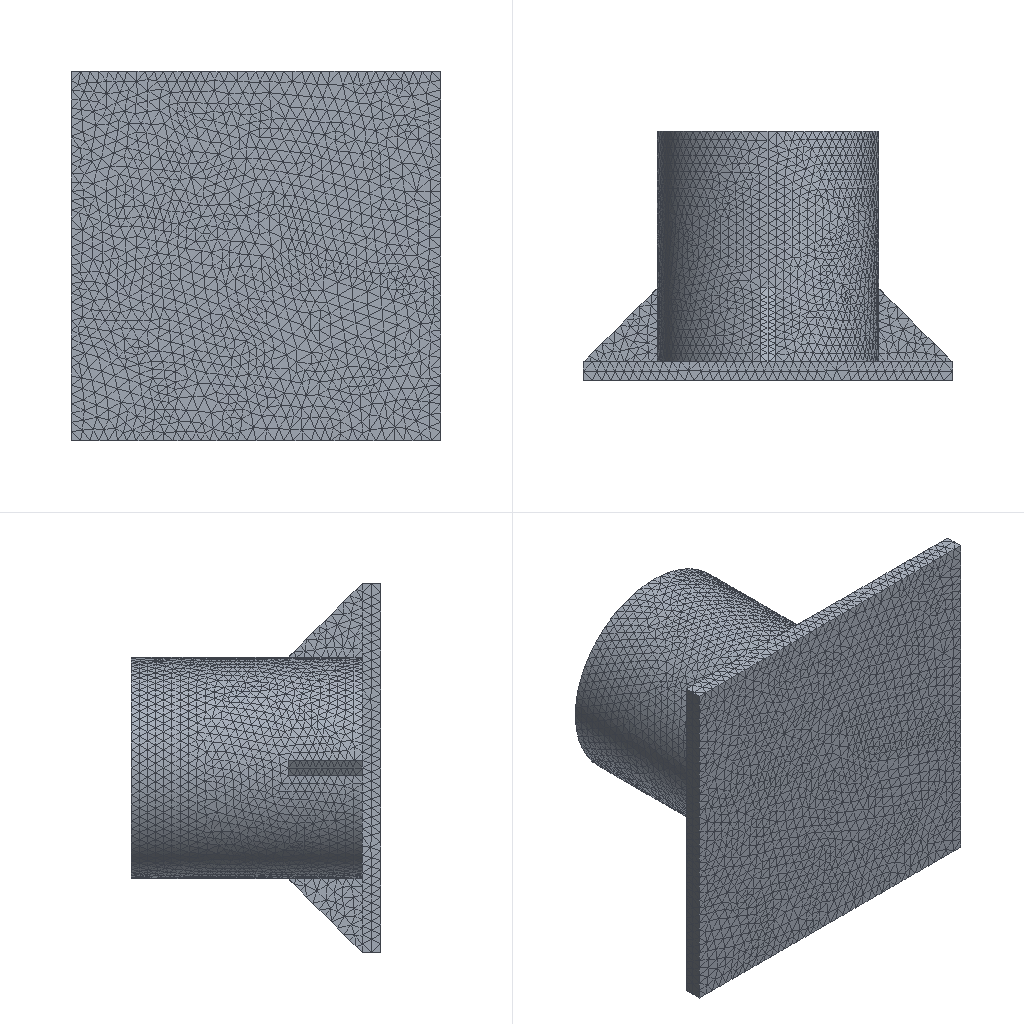Simulation study | ansys workbench
Set-up summary:
category,name,step,type,value,unit,region
solver,ansys_workbench
units,mm-N-s-tonne (MPa),,stated,"/units,MPA"
analysis,LS1,,modal,method=lanb; n_modes=3
load_step,LS1,LS1,modal
mesh,nodes,,,70254
mesh,elements,,,42512
element_type,SOLID187,,,41872
element_type,CONTA174,,,640
material,Structural Steel,,E,200000,tonne s^-2 mm^-1
material,Structural Steel,,nu,0.3
material,Structural Steel,,density,7.8e-09,tonne mm^-3
bc,Construct Remote Displacement,model,fixed,"[dofs=ROTX,ROTY,ROTZ,UX,UY,UZ n=20]",,node list
contact,contact 1,,bonded (always),element=CONTA174
contact,contact 2,,bonded (always),element=CONTA174
contact,contact 3,,bonded (always),element=CONTA174
contact,contact 4,,bonded (always),element=CONTA174
named_set,REMOTEDISPALL,,node,4
Ansys APDL input file, long lists of numbers shortened:
/batch
/config,noeldb,1     ! force off writing results to database
*get,_wallstrt,active,,time,wall
! ANSYS input file written by Workbench version 2021 R1
! File used for geometry attach:
/title,wbnew--__ (C5)
! ****** Begin Custom Load Command Snippet ******
/COM, ACT Extensions:
/COM,     LSDYNA, 2021.1
/COM,
! ****** End   Custom Load Command Snippet ******
*DIM,_wb_ProjectScratch_dir,string,248
_wb_ProjectScratch_dir(1) = ''
*DIM,_wb_SolverFiles_dir,string,248
_wb_SolverFiles_dir(1) = ''
*DIM,_wb_userfiles_dir,string,248
_wb_userfiles_dir(1) = ''
/com,--- Data in consistent NMM units. See Solving Units in the help system for more information.
/units,MPA
/nopr
/wb,file,start              !  signify a WB generated input file
/prep7
! Turn off shape checking because checks already performed inside WB mesher.
! See help system for more information.
SHPP,OFF,,NOWARN
/nolist
etcon,set             ! allow ANSYS to choose best KEYOP's for 180x elements, resets any applicable keyopt to MAPDL defaults
/com,*********** Nodes for the whole assembly ***********
nblock,3,,77270
(1i9,3e20.9e3)
        1     0.000000000E+00     2.700000000E+03    -1.000000000E+03
! (70245 more lines like these left out)
-1
/com,*********** Nodes for all Remote Points ***********
nblock,3
(1i9,3e20.9e3)
    70247    -2.000000000E+03     1.000000000E+02    -3.725290298E-14
! (7 more lines like these left out)
-1
/wb,elem,start            !  set before creation of elements
/com,*********** Elements for Body 1 "__-FreeParts|____(____)1" ***********
et,1,187
eblock,19,solid,,41872
(19i9)
        1        1        1        1        0        0        0        0       10        0        1     8226    10631     9051     9803    64966    68065    64961    64962
! (83743 more lines like these left out)
-1
/wb,elem,end               !  done creating elements
/com,*********** Send User Defined Coordinate System(s) ***********
csys,0
toffst,273.15,  ! Temperature offset from absolute zero
/com,*********** Set Reference Temperature ***********
tref,22.
/wb,mat,start              !  starting to send materials
/com,*********** Send Materials ***********
MP,DENS,1,7.8e-09,	! tonne mm^-3
MP,EX,1,200000,	! tonne s^-2 mm^-1
MP,NUXY,1,0.3,
/wb,mat,end                !  done sending materials
!************************* Model Summary ********************
!__-FreeParts|____(____)1,	结构钢,	matid,	1
!************************* End Model Summary ********************
! get the diagonal of the bounding box. Needed later for other things
*get,_xmin,node,,mnloc,x
*get,_ymin,node,,mnloc,y
*get,_zmin,node,,mnloc,z
*get,_xmax,node,,mxloc,x
*get,_ymax,node,,mxloc,y
*get,_zmax,node,,mxloc,z
_ASMDIAG=(_xmax-_xmin)*(_xmax-_xmin)+(_ymax-_ymin)*(_ymax-_ymin)+(_zmax-_zmin)*(_zmax-_zmin)
_ASMDIAG=SQRT(_ASMDIAG)
/wb,contact,start          !  starting to send contact
/wb,contact,end            !  done creating contacts
/golist
/wb,load,start             !  starting to send loads
/com,*********** Create Remote Point "内部远程点 5" ***********
! -------- Remote Point Used by "远程位移" --------
*set,tid,3
*set,cid,2
et,cid,174
et,tid,170
keyo,tid,2,1               ! Don't fix the pilot node
keyo,tid,4,111111
keyo,cid,12,5              ! Bonded Contact
keyo,cid,4,1               ! Deformable RBE3 style load
keyo,cid,2,2               ! MPC style contact
eblock,10,,,160
(15i9)
    56107        2        2        2        0      379     4570      380      380    13806    13810      380    13803
! (159 more lines like these left out)
-1
*set,_npilot,70251
_npilot55=_npilot
type,tid
mat ,cid
real,cid
tshape,pilo
en,56267,_npilot
tshape
/com,*********** Create Remote Point "内部远程点 5" ***********
! -------- Remote Point Used by "远程位移 2" --------
*set,tid,5
*set,cid,4
et,cid,174
et,tid,170
keyo,tid,2,1               ! Don't fix the pilot node
keyo,tid,4,111111
keyo,cid,12,5              ! Bonded Contact
keyo,cid,4,1               ! Deformable RBE3 style load
keyo,cid,2,2               ! MPC style contact
eblock,10,,,160
(15i9)
    56268        4        4        4        0      455      456     4685     4685    14423    14430     4685    14426
! (159 more lines like these left out)
-1
*set,_npilot,70252
_npilot58=_npilot
type,tid
mat ,cid
real,cid
tshape,pilo
en,56428,_npilot
tshape
/com,*********** Create Remote Point "内部远程点 5" ***********
! -------- Remote Point Used by "远程位移 3" --------
*set,tid,7
*set,cid,6
et,cid,174
et,tid,170
keyo,tid,2,1               ! Don't fix the pilot node
keyo,tid,4,111111
keyo,cid,12,5              ! Bonded Contact
keyo,cid,4,1               ! Deformable RBE3 style load
keyo,cid,2,2               ! MPC style contact
eblock,10,,,160
(15i9)
    56429        6        6        6        0      264     4645      559      559    12988    15049      559    12986
! (159 more lines like these left out)
-1
*set,_npilot,70253
_npilot61=_npilot
type,tid
mat ,cid
real,cid
tshape,pilo
en,56589,_npilot
tshape
/com,*********** Create Remote Point "内部远程点 5" ***********
! -------- Remote Point Used by "远程位移 4" --------
*set,tid,9
*set,cid,8
et,cid,174
et,tid,170
keyo,tid,2,1               ! Don't fix the pilot node
keyo,tid,4,111111
keyo,cid,12,5              ! Bonded Contact
keyo,cid,4,1               ! Deformable RBE3 style load
keyo,cid,2,2               ! MPC style contact
eblock,10,,,160
(15i9)
    56590        8        8        8        0      538      561     4608     4608    14920    15056     4608    14922
! (159 more lines like these left out)
-1
*set,_npilot,70254
_npilot64=_npilot
type,tid
mat ,cid
real,cid
tshape,pilo
en,56750,_npilot
tshape
/com,*********** Construct Remote Displacement ***********
*DIM,_loadvari54ux,TABLE,1,1,1,TIME,
! Time values
_loadvari54ux(1,0,1) = 1.
! Load values
_loadvari54ux(1,1,1) = 0.
*DIM,_loadvari54uy,TABLE,1,1,1,TIME,
! Time values
_loadvari54uy(1,0,1) = 1.
! Load values
_loadvari54uy(1,1,1) = 0.
*DIM,_loadvari54uz,TABLE,1,1,1,TIME,
! Time values
_loadvari54uz(1,0,1) = 1.
! Load values
_loadvari54uz(1,1,1) = 0.
*DIM,_loadvari54roty,TABLE,1,1,1,TIME,
! Time values
_loadvari54roty(1,0,1) = 1.
! Load values
_loadvari54roty(1,1,1) = 0.
*DIM,_loadvari54rotz,TABLE,1,1,1,TIME,
! Time values
_loadvari54rotz(1,0,1) = 1.
! Load values
_loadvari54rotz(1,1,1) = 0.
/com,*********** Construct Remote Displacement ***********
*DIM,_loadvari57ux,TABLE,1,1,1,TIME,
! Time values
_loadvari57ux(1,0,1) = 1.
! Load values
_loadvari57ux(1,1,1) = 0.
*DIM,_loadvari57uy,TABLE,1,1,1,TIME,
! Time values
_loadvari57uy(1,0,1) = 1.
! Load values
_loadvari57uy(1,1,1) = 0.
*DIM,_loadvari57uz,TABLE,1,1,1,TIME,
! Time values
_loadvari57uz(1,0,1) = 1.
! Load values
_loadvari57uz(1,1,1) = 0.
*DIM,_loadvari57rotx,TABLE,1,1,1,TIME,
! Time values
_loadvari57rotx(1,0,1) = 1.
! Load values
_loadvari57rotx(1,1,1) = 0.
*DIM,_loadvari57roty,TABLE,1,1,1,TIME,
! Time values
_loadvari57roty(1,0,1) = 1.
! Load values
_loadvari57roty(1,1,1) = 0.
/com,*********** Construct Remote Displacement ***********
*DIM,_loadvari60ux,TABLE,1,1,1,TIME,
! Time values
_loadvari60ux(1,0,1) = 1.
! Load values
_loadvari60ux(1,1,1) = 0.
*DIM,_loadvari60uy,TABLE,1,1,1,TIME,
! Time values
_loadvari60uy(1,0,1) = 1.
! Load values
_loadvari60uy(1,1,1) = 0.
*DIM,_loadvari60uz,TABLE,1,1,1,TIME,
! Time values
_loadvari60uz(1,0,1) = 1.
! Load values
_loadvari60uz(1,1,1) = 0.
*DIM,_loadvari60roty,TABLE,1,1,1,TIME,
! Time values
_loadvari60roty(1,0,1) = 1.
! Load values
_loadvari60roty(1,1,1) = 0.
*DIM,_loadvari60rotz,TABLE,1,1,1,TIME,
! Time values
_loadvari60rotz(1,0,1) = 1.
! Load values
_loadvari60rotz(1,1,1) = 0.
/com,*********** Construct Remote Displacement ***********
*DIM,_loadvari63ux,TABLE,1,1,1,TIME,
! Time values
_loadvari63ux(1,0,1) = 1.
! Load values
_loadvari63ux(1,1,1) = 0.
*DIM,_loadvari63uy,TABLE,1,1,1,TIME,
! Time values
_loadvari63uy(1,0,1) = 1.
! Load values
_loadvari63uy(1,1,1) = 0.
*DIM,_loadvari63uz,TABLE,1,1,1,TIME,
! Time values
_loadvari63uz(1,0,1) = 1.
! Load values
_loadvari63uz(1,1,1) = 0.
*DIM,_loadvari63rotx,TABLE,1,1,1,TIME,
! Time values
_loadvari63rotx(1,0,1) = 1.
! Load values
_loadvari63rotx(1,1,1) = 0.
*DIM,_loadvari63roty,TABLE,1,1,1,TIME,
! Time values
_loadvari63roty(1,0,1) = 1.
! Load values
_loadvari63roty(1,1,1) = 0.
d,70251,ux,%_loadvari54ux%
d,70251,uy,%_loadvari54uy%
d,70251,uz,%_loadvari54uz%
d,70251,roty,%_loadvari54roty%
d,70251,rotz,%_loadvari54rotz%
d,70252,ux,%_loadvari57ux%
d,70252,uy,%_loadvari57uy%
d,70252,uz,%_loadvari57uz%
d,70252,rotx,%_loadvari57rotx%
d,70252,roty,%_loadvari57roty%
d,70253,ux,%_loadvari60ux%
d,70253,uy,%_loadvari60uy%
d,70253,uz,%_loadvari60uz%
d,70253,roty,%_loadvari60roty%
d,70253,rotz,%_loadvari60rotz%
d,70254,ux,%_loadvari63ux%
d,70254,uy,%_loadvari63uy%
d,70254,uz,%_loadvari63uz%
d,70254,rotx,%_loadvari63rotx%
d,70254,roty,%_loadvari63roty%
/COM,*** Create a component for all remote displacements ***
CMBLOCK,REMOTEDISPALL,NODE,        4
(8i10)
     70251     70252     70253     70254
/gst,on,on
fini
*get,_numnode,node,0,count
*get,_numelem,elem,0,count
*get, _MAXELEMNUM, elem, 0, NUM, MAX
*get, _MAXNODENUM, node, 0, NUM, MAX
*get, _MAXELEMTYPE, etyp, 0, NUM, MAX
*get, _MAXREALCONST, real, 0, NUM, MAX
/go
/wb,load,end               !  done creating loads
/com,--- Number of total nodes = %_numnode%
/com,--- Number of contact elements = 640
/com,--- Number of spring elements = 0
/com,--- Number of bearing elements = 0
/com,--- Number of solid elements = 41872
/com,--- Number of condensed parts = 0
/com,--- Number of total elements = %_numelem%
*get,_wallbsol,active,,time,wall
/solu
antype,2                   ! modal analysis
_thickRatio=  1     ! Ratio of thick parts in the model
modopt,lanb,3
outres,erase
outres,all,none
outres,nsol,all
outres,etmp,all
mxpand                    ! default expand in case of complex solution
dmpopt,esav,no
dmpopt,emat,no
dmpopt,full,no
! *********** WB SOLVE COMMAND ***********
! check interactive state
*get,ANSINTER_,active,,int
*if,ANSINTER_,ne,0,then
/eof
*endif
solve
/com *************** Write FE CONNECTORS *********
CEWRITE,file,ce,,INTE
*get,_nmodalsolproc,active,0,numcpu
fini
/nopr
*get,_numnode,node,0,count
*get,_numelem,elem,0,count
*get, _MAXELEMNUM, elem, 0, NUM, MAX
*get, _MAXNODENUM, node, 0, NUM, MAX,,,INTERNAL
*get, _MAXELEMTYPE, etyp, 0, NUM, MAX
*get, _MAXREALCONST, real, 0, NUM, MAX
/gopr
*get,_wallasol,active,,time,wall
/post1
/nopr
*dim,_direction,CHAR,6,1
_direction(1) = 'X'
_direction(2) = 'Y'
_direction(3) = 'Z'
_direction(4) = 'ROTX'
_direction(5) = 'ROTY'
_direction(6) = 'ROTZ'
*get,_lastLS,active,0,set,LSTP
*get,_beginset,active,0,set,nset,first,_lastLS
*get,_endset,active,0,set,nset,last,_lastLS
_nummodes = 0
*if,_endset,gt,0,then
_nummodes = _endset - _beginset + 1
*endif
*do,i_mode,1,_nummodes
   *do,j_component,1,6
			*get,PFACT_%i_mode%_%j_component%,MODE,%i_mode%,PFACT,,DIREC,_direction(%j_component%)
   *enddo
*enddo
*dim,_tmdirection,CHAR,6,1
_tmdirection(1) = 'X'
_tmdirection(2) = 'Y'
_tmdirection(3) = 'Z'
_tmdirection(4) = 'X'
_tmdirection(5) = 'Y'
_tmdirection(6) = 'Z'
*do,j_component,1,6
    *if,j_component,gt,3,then
        *get,TOTALMASS_%j_component%,ELEM,0,IOR,_tmdirection(%j_component%)
    *else
        *get,TOTALMASS_%j_component%,ELEM,0,MTOT,_tmdirection(%j_component%)
    *endif
*enddo
/gopr
xmlo,ENCODING,ISO-8859-1
xmlo,parm
/xml,parm,xml
fini
/gopr
*get,_walldone,active,,time,wall
_preptime=(_wallbsol-_wallstrt)*3600
_solvtime=(_wallasol-_wallbsol)*3600
_posttime=(_walldone-_wallasol)*3600
_totaltim=(_walldone-_wallstrt)*3600
*get,_dlbratio,active,0,solu,dlbr
*get,_combtime,active,0,solu,comb
/com,--- Total number of nodes = %_numnode%
/com,--- Total number of elements = %_numelem%
/com,--- Element load balance ratio = %_dlbratio%
/com,--- Time to combine distributed files = %_combtime%
/wb,file,end               ! done with WB generated input
Results summary:
result,analyses[0].index,,,1
result,analyses[0].system,,,SYS-2
result,analyses[0].deck,,,deck.dat
result,analyses[0].solve_status,,,completed
result,analyses[0].analysis_type,,,modal
result,analyses[0].physics,,,mechanical
result,analyses[0].unit_system,,,"NMM: mm, ton, N, s, mV, mA, degC"
result,analyses[0].n_sets,,,3
result,analyses[0].modal_frequencies_hz[1],,,20.581
result,analyses[0].modal_frequencies_hz[2],,,24.283
result,analyses[0].modal_frequencies_hz[3],,,47.376
result,geometry_export[0][0],,,.step
result,geometry_export[0][1],,,ok
result,geometry_export[0][2],,,1